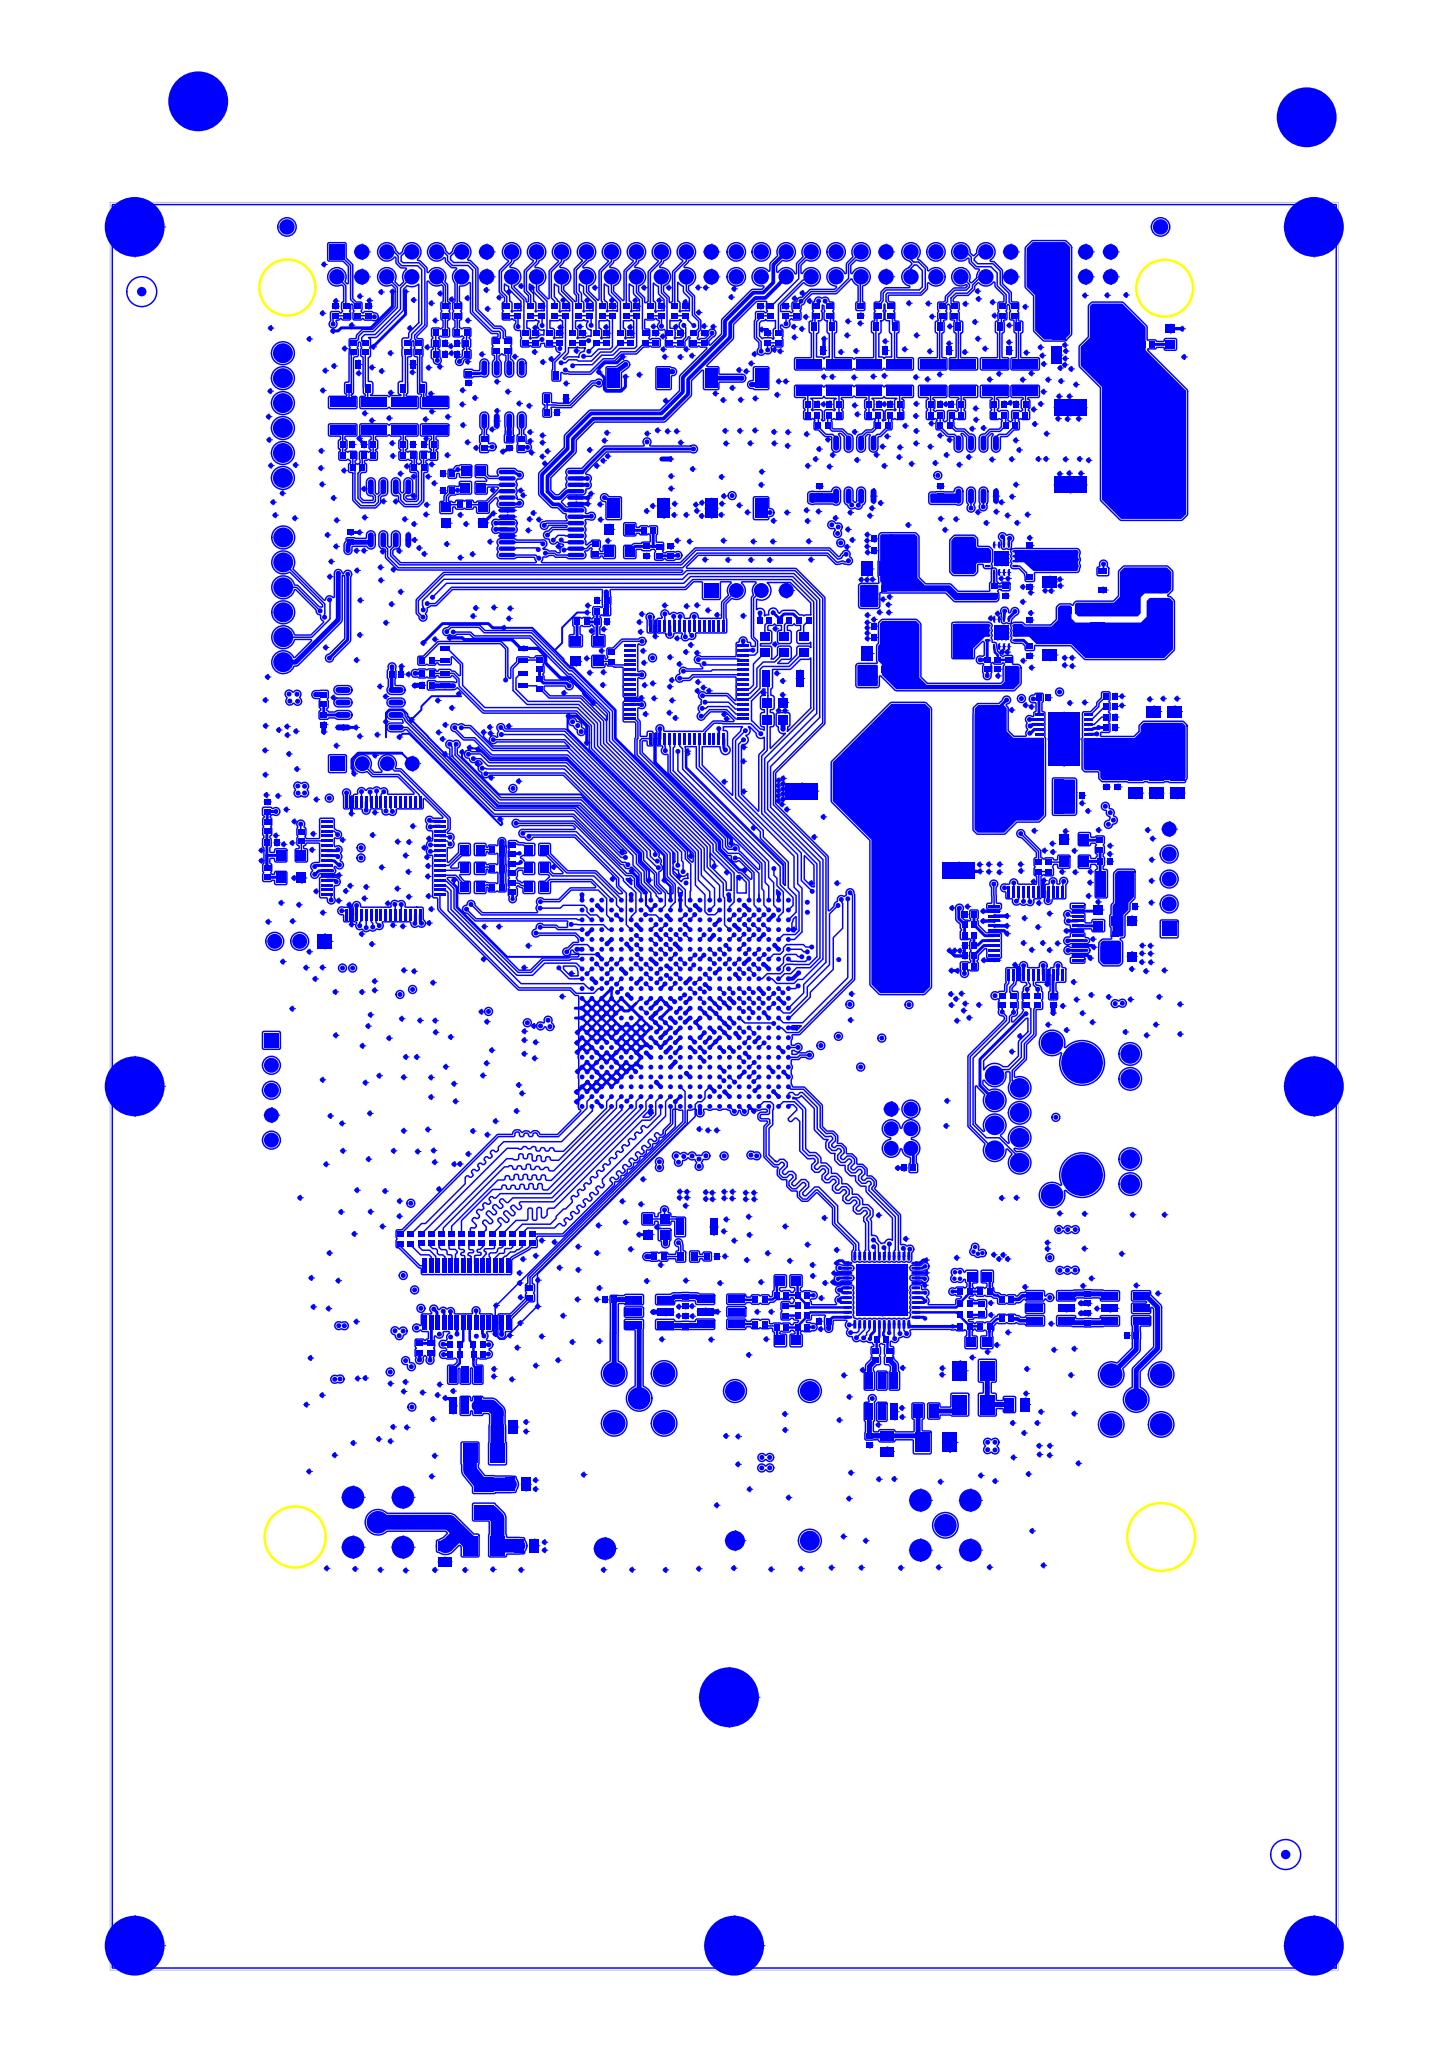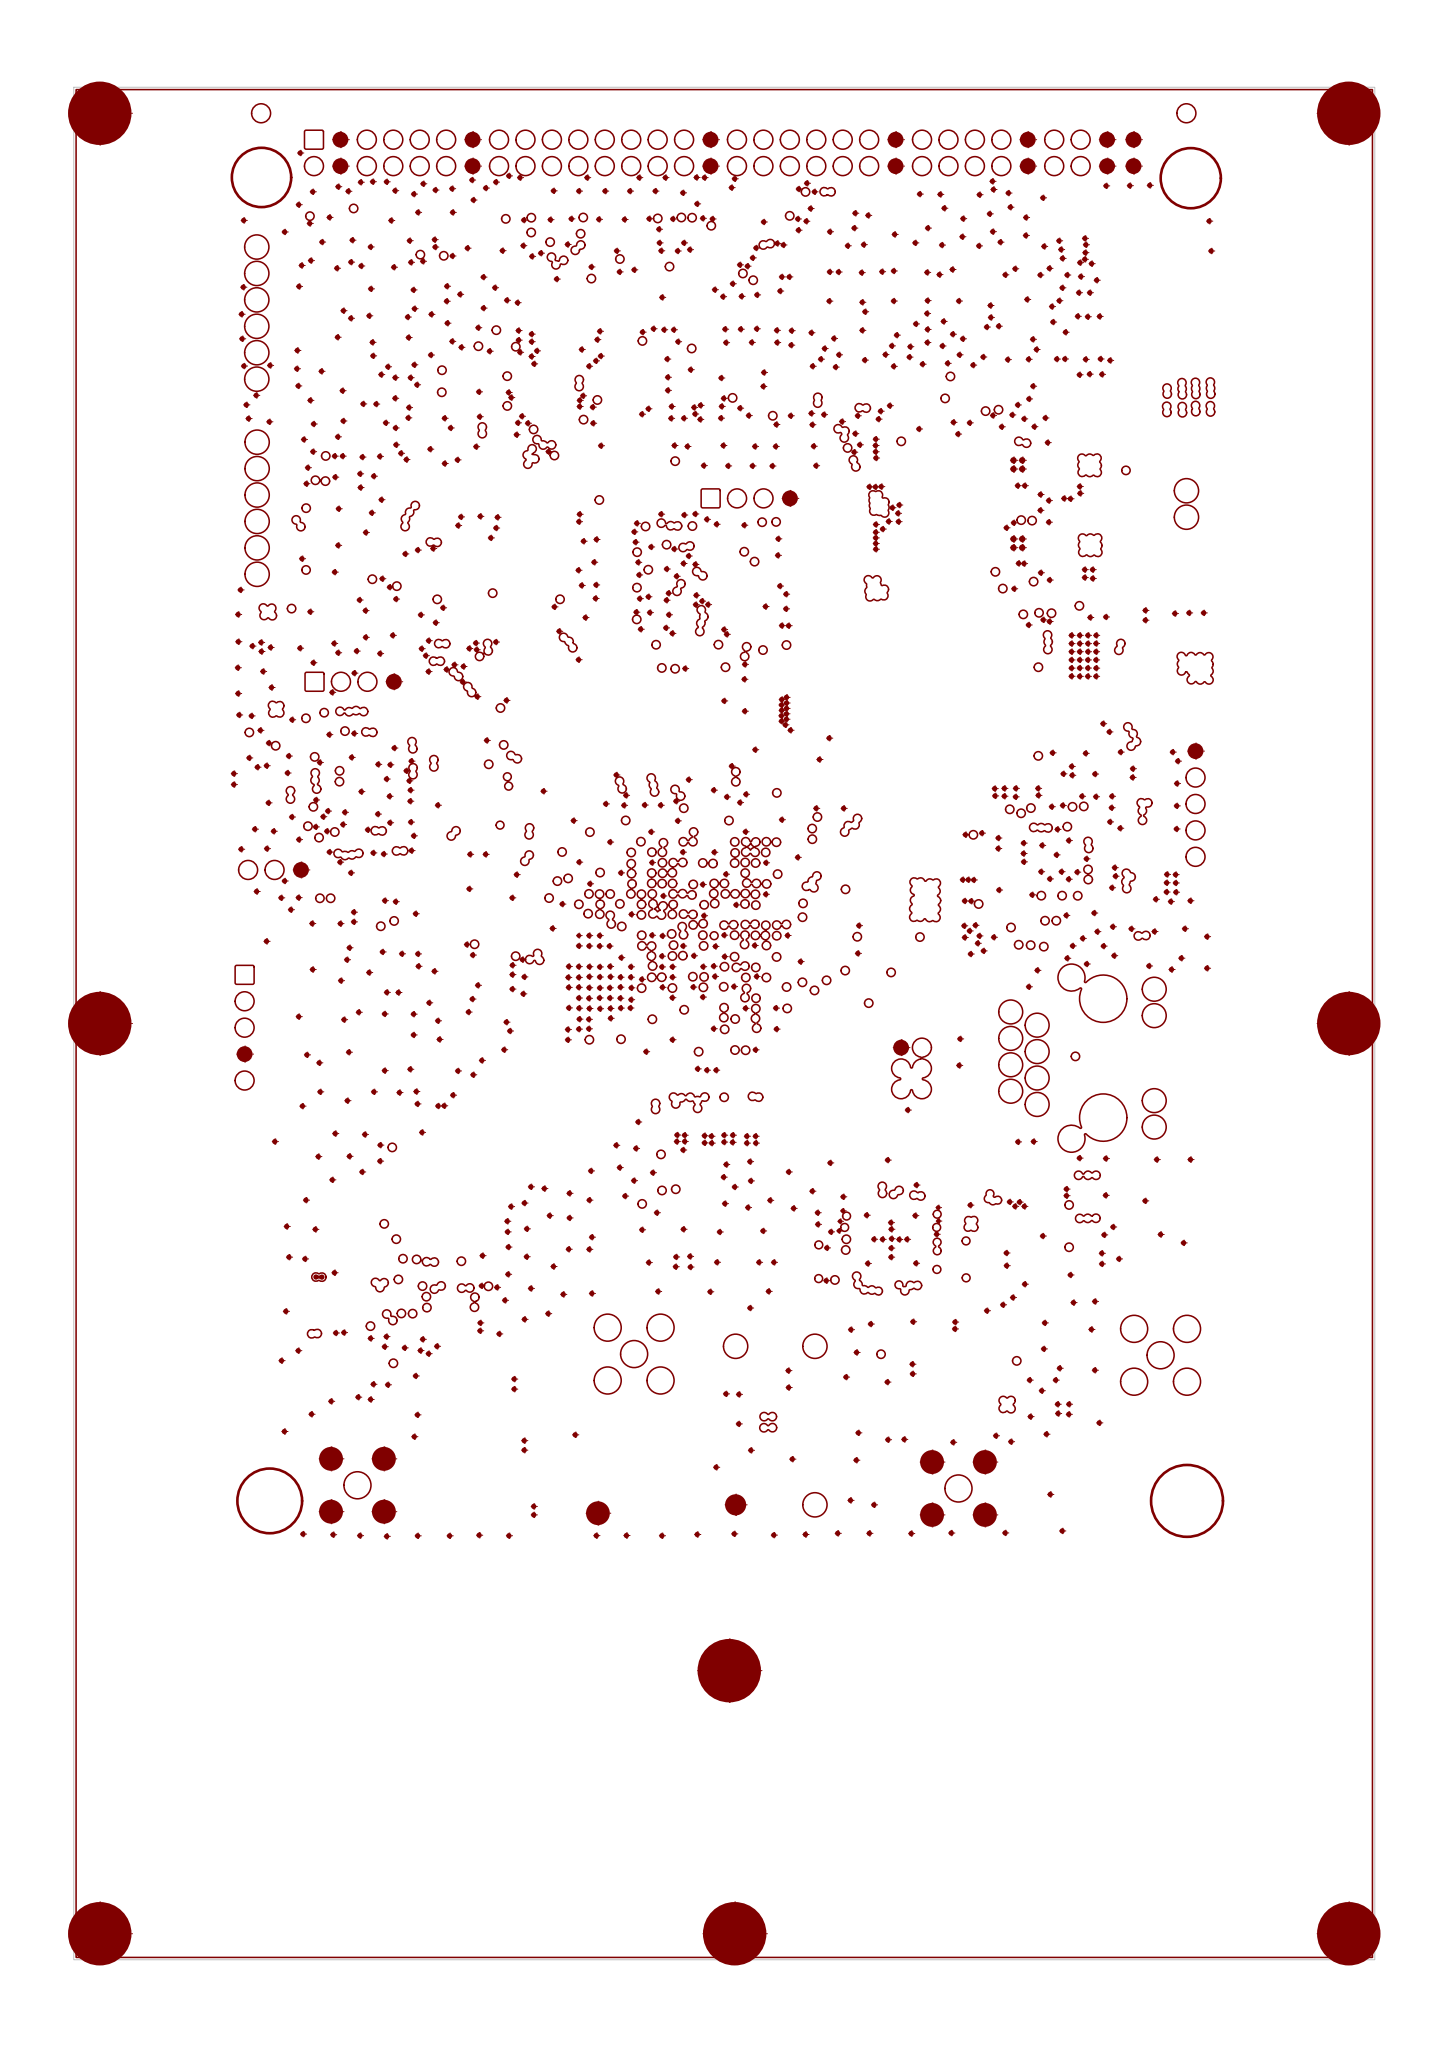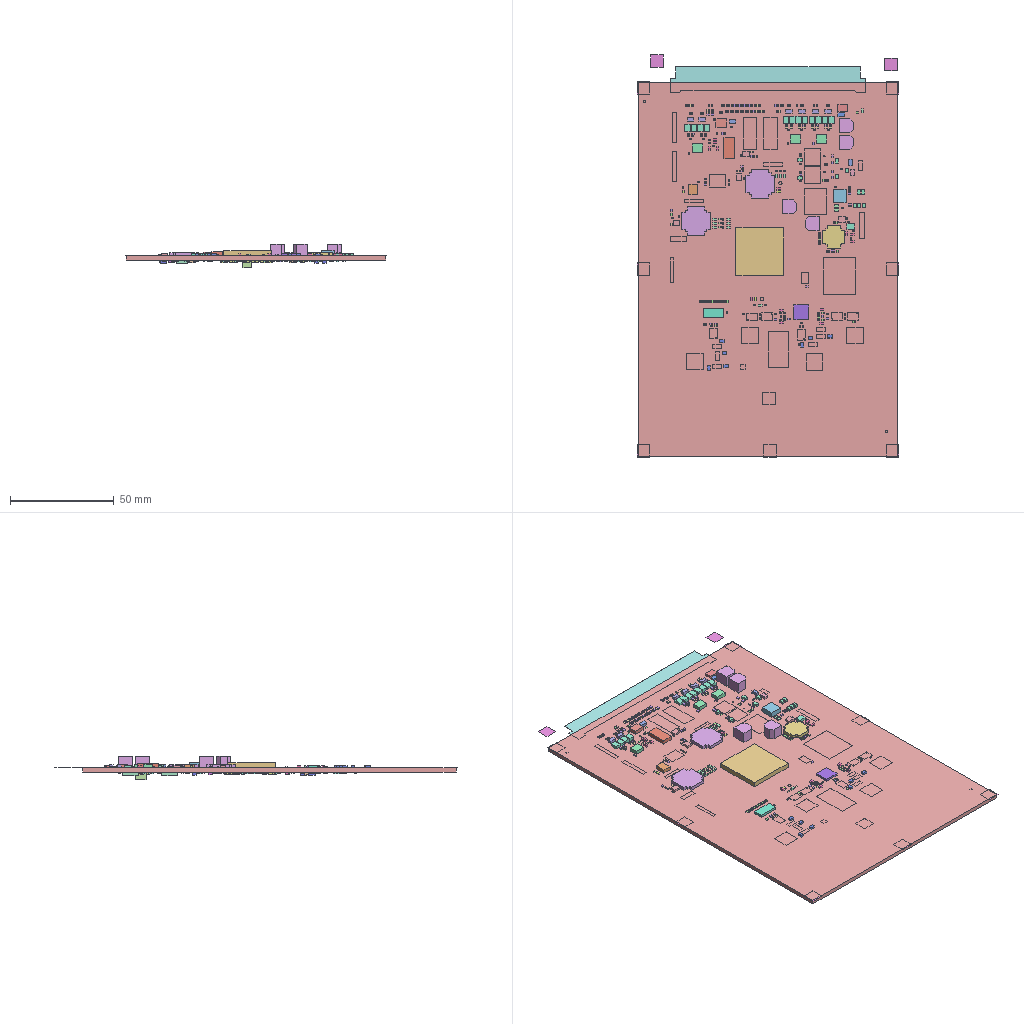Circuit board layout | Siemens PADS | box 126.1 x 193.9 x 11.1 mm
Layer stack:
layer,name,type,plane,layer_thickness_mm,copper_thickness_mm,dielectric_constant
0,,,,0,,3.3
1,Top,ROUTING,NONE,0.283,0.034,4.3
2,GND2,ROUTING,NONE,0.254,0.0351,4.3
3,SIG3,ROUTING,NONE,0.554,0.034,4.3
4,SIG4,ROUTING,NONE,0.2499,0.034,4.3
5,POWER5,ROUTING,NONE,0.4539,0.034,4.3
6,Bottom,ROUTING,NONE,0,0.034,3.3
Part placement, first 430 of 633 lines:
Ref,PartType,Decal,X_mm,Y_mm,Rotation,Layer,Placed,Installed
C1,CAP0805,CAPC1005X60N,30.658,-36.805,270,Bottom,True,True
C2,CAP0805,CAPC1005X60N,32.514,-101.452,270,Bottom,True,True
C3,CAP0805,CAPC2013X100L,40.208,-124.689,0,Top,True,True
C4,CAP0805,CAPC2013X100L,41.504,-130.531,0,Top,True,True
C5,CAP0805,CAPC2013X100L,42.367,-136.779,0,Top,True,True
C6,CAP0805,CAPC1608X90N,28.514,-117.318,90,Bottom,True,True
C7,CAP0805,CAPC1005X60N,70.622,-131.846,180,Bottom,True,True
C8,CAP0805,CAPC1005X60N,81.579,-126.895,270,Bottom,True,True
C9,CAP0805,CAPC1005X60N,77.069,-122.882,0,Bottom,True,True
C10,CAP0805,CAPC1005X60N,76.578,-131.624,270,Bottom,True,True
C11,CAP0805,CAPC2013X100L,92.32,-122.4,0,Top,True,True
C12,CAP0805,CAPC1608X90N,70.325,-123.37,180,Bottom,True,True
C13,CAP0805,CAPC1608X90N,70.336,-124.988,180,Bottom,True,True
C14,CAP0805,CAPC1608X90N,83.129,-126.57,270,Bottom,True,True
C15,CAP0805,CAPC1005X60N,88.724,-112.651,270,Top,True,True
C16,CAP0805,CAPC1005X60N,86.97,-114.46,0,Bottom,True,True
C17,CAP0805,CAPC1005X60N,91.239,-111.702,180,Top,True,True
C18,CAP0805,CAPC1608X90N,28.514,-121.876,270,Bottom,True,True
C19,CAP0805,CAPC1005X60N,30.067,-122.17,90,Bottom,True,True
C20,CAP0805,CAPC1005X60N,30.067,-116.806,270,Bottom,True,True
C21,CAP0805,CAPC1005X60N,32.527,-114.113,270,Bottom,True,True
C22,CAP0805,CAPC1005X60N,34.647,-114.113,270,Bottom,True,True
C23,CAP0805,CAPC1005X60N,37.277,-114.113,270,Bottom,True,True
C24,CAP0805,CAPC1005X60N,35.086,-116.297,180,Top,True,True
C25,CAP0805,CAPC1005X60N,37.466,-116.297,0,Top,True,True
C26,CAP0805,CAPC1608X90N,88.59,-27.07,270,Bottom,True,True
C27,CAP0805,CAPC1005X60N,87.157,-27.306,90,Bottom,True,True
C28,CAP0805,CAPC1005X60N,94.751,-27.414,90,Bottom,True,True
C29,CAP0805,CAPC2013X100L,34.036,-137.617,270,Top,True,True
C30,CAP0805,CAPC1005X60N,91.239,-113.684,180,Top,True,True
C31,CAP-AE4,CAPAE660X550N,100.29,-20.91,180,Top,True,True
C32,CAP0805,CAPC1005X60N,68.775,-11.06,270,Top,True,True
C33,CAP0805,CAPC1005X60N,54.57,-35.52,90,Top,True,True
C34,CAP0805,CAPC1005X60N,57.04,-35.52,270,Top,True,True
C35,CAP0805,CAPC1608X90N,54.76,-104.3,90,Top,True,True
C36,CAP0805,CAPC1005X60N,32.23,-49.174,180,Top,True,True
C37,CAP0805,CAPC1005X60N,98.675,-73.229,180,Bottom,True,True
C38,CAP0805,CAPC1005X60N,98.675,-75.007,180,Bottom,True,True
C39,CAP0805,CAPC1005X60N,55.43,-43.03,0,Bottom,True,True
C40,CAP0805,CAPC1005X60N,64.42,-43.38,270,Bottom,True,True
C41,CAP0805,CAPC1005X60N,52.783,-48.135,180,Bottom,True,True
C42,CAP0805,CAPC1005X60N,50.03,-42.72,180,Top,True,True
C43,CAP0805,CAPC1005X60N,50.03,-40.53,0,Top,True,True
C44,CAP0805,CAPC1005X60N,64.18,-45.59,180,Bottom,True,True
C45,CAP0805,CAPC1005X60N,61.21,-54.52,180,Bottom,True,True
C46,CAP0805,CAPC1005X60N,52.825,-51.147,180,Bottom,True,True
C47,CAP0805,CAPC1005X60N,63.18,-54.54,0,Bottom,True,True
C48,CAP0805,CAPC1608X90N,62.33,-43.84,180,Bottom,True,True
C49,CAP0805,CAPC1005X60N,84.462,-29.402,270,Top,True,True
C50,CAP0805,CAPC1005X60N,72.165,-29.402,270,Top,True,True
C51,CAP0805,CAPC1005X60N,73.681,-20.551,180,Top,True,True
C52,CAP0805,CAPC1005X60N,55.44,-54.57,180,Bottom,True,True
C53,CAP0805,CAPC1005X60N,71.491,-20.551,0,Top,True,True
C54,CAP0805,CAPC1005X60N,68.751,-112.863,270,Top,True,True
C55,CAP0805,CAPC1005X60N,77.917,-117.419,90,Top,True,True
C56,CAP0805,CAPC1005X60N,79.27,-117.419,90,Top,True,True
C57,CAP0805,CAPC1005X60N,79.854,-20.551,180,Top,True,True
C58,CAP0805,CAPC1005X60N,77.714,-20.551,0,Top,True,True
C59,CAP0805,CAPC1005X60N,24.497,-34.095,270,Top,True,True
C60,CAP0805,CAPC1005X60N,24.16,-24.657,0,Top,True,True
C61,CAP0805,CAPC1005X60N,26.3,-24.657,180,Top,True,True
C62,CAP0805,CAPC1005X60N,30.315,-24.657,0,Top,True,True
C63,CAP0805,CAPC1005X60N,32.445,-24.657,180,Top,True,True
C64,CAP0805,CAPC2013X100L,83.025,-123.064,0,Top,True,True
C65,CAP0805,CAPC2013X100L,79.046,-126.389,270,Top,True,True
C66,CAP0805,CAPC1005X60N,66.9,-13.81,270,Top,True,True
C67,CAP0805,CAPC1005X60N,56.087,-11.06,270,Top,True,True
C68,CAP0805,CAPC1005X60N,74.98,-110.03,270,Bottom,True,True
C69,CAP0805,CAPC1005X60N,74.98,-107.93,90,Bottom,True,True
C70,CAP0805,CAPC1005X60N,82,-107.96,90,Bottom,True,True
C71,CAP0805,CAPC1005X60N,82,-110.02,270,Bottom,True,True
C72,CAP0805,CAPC1005X60N,89.844,-110.018,270,Bottom,True,True
C73,CAP0805,CAPC1005X60N,98.233,-110.079,270,Bottom,True,True
C74,CAP0805,CAPC1608X90N,92.388,-110.297,90,Bottom,True,True
C75,CAP0805,CAPC1005X60N,90.96,-105.941,270,Bottom,True,True
C76,CAP0805,CAPC1005X60N,98.233,-106.056,270,Bottom,True,True
C77,CAP0805,CAPC1608X90N,92.388,-106.248,90,Bottom,True,True
C78,CAP0805,CAPC1005X60N,98.675,-76.082,180,Bottom,True,True
C79,CAP0805,CAPC1005X60N,96.391,-76.62,90,Bottom,True,True
C80,CAP0805,CAPC1005X60N,94.891,-76.62,90,Bottom,True,True
C81,CAP0805,CAPC1005X60N,92.933,-76.62,90,Bottom,True,True
C82,CAP0805,CAPC1608X90N,103.16,-73.154,180,Top,True,True
C83,CAP0805,CAPC1005X60N,98.675,-72.14,180,Bottom,True,True
C84,CAP0805,CAPC1608X90N,100.558,-72.842,270,Top,True,True
C85,CAP0805,CAPC1005X60N,101.239,-67.1,180,Top,True,True
C86,CAP0805,CAPC1005X60N,103.808,-71.702,180,Top,True,True
C87,CAP0805,CAPC1005X60N,95,-70.37,0,Bottom,True,True
C88,CAP0805,CAPC1005X60N,95.77,-95.24,0,Bottom,True,True
C89,CAP0805,CAPC1005X60N,93.296,-81.246,270,Top,True,True
C90,CAP0805,CAPC1005X60N,94.424,-81.246,270,Top,True,True
C91,CAP0805,CAPC1005X60N,86.382,-91.479,0,Bottom,True,True
C92,CAP0805,CAPC1608X90N,103.16,-76.79,180,Top,True,True
C93,CAP0805,CAPC1005X60N,58.543,-11.06,270,Top,True,True
C94,CAP0805,CAPC1005X60N,58.024,-13.81,270,Top,True,True
C95,CAP0805,CAPC1005X60N,86.112,-20.551,180,Top,True,True
C96,CAP0805,CAPC1005X60N,60.454,-13.81,270,Top,True,True
C97,CAP0805,CAPC1005X60N,55.51,-13.81,270,Top,True,True
C98,CAP0805,CAPC1005X60N,53.582,-11.06,270,Top,True,True
C99,CAP0805,CAPC1005X60N,83.982,-20.551,0,Top,True,True
C100,CAP0805,CAPC1005X60N,52.989,-13.81,270,Top,True,True
C101,CAP0805,CAPC1005X60N,92.668,-20.551,180,Top,True,True
C102,CAP0805,CAPC1005X60N,90.487,-20.551,0,Top,True,True
C103,CAP0805,CAPC1005X60N,51.119,-11.06,270,Top,True,True
C104,CAP0805,CAPC1608X90N,99.43,-54.92,90,Bottom,True,True
C105,CAP0805,CAPC1608X90N,101.73,-54.26,90,Bottom,True,True
C106,CAP0805,CAPC1005X60N,101.803,-53.491,0,Top,True,True
C107,CAP0805,CAPC1005X60N,50.543,-13.81,270,Top,True,True
C108,CAP0805,CAPC1005X60N,48.752,-11.06,270,Top,True,True
C109,CAP0805,CAPC1005X60N,48.09,-13.81,270,Top,True,True
C110,CAP0805,CAPC1005X60N,46.341,-11.06,270,Top,True,True
C111,CAP0805,CAPC1005X60N,45.72,-13.81,270,Top,True,True
C112,CAP0805,CAPC1005X60N,23.719,-37.168,180,Bottom,True,True
C113,CAP0805,CAPC1005X60N,63.897,-124.312,270,Bottom,True,True
C114,CAP0805,CAPC1005X60N,43.872,-11.06,270,Top,True,True
C115,CAP0805,CAPC1005X60N,43.328,-13.81,270,Top,True,True
C116,CAP0805,CAPC1005X60N,22.904,-11.06,270,Top,True,True
C117,CAP0805,CAPC1005X60N,41.45,-11.06,270,Top,True,True
C118,CAP0805,CAPC1005X60N,26.278,-11.06,270,Top,True,True
C119,CAP0805,CAPC1005X60N,66.16,-11.06,270,Top,True,True
C120,CAP0805,CAPC1005X60N,104.883,-71.281,0,Bottom,True,True
C121,CAP0805,CAPC1005X60N,104.883,-69.086,0,Bottom,True,True
C122,CAP0805,CAPC1005X60N,104.883,-66.89,0,Bottom,True,True
C123,CAP0805,CAPC2013X120N,106.21,-52.745,90,Top,True,True
C124,CAP0805,CAPC2013X120N,108.577,-59.248,270,Top,True,True
C125,CAP0805,CAPC2013X120N,106.44,-59.248,270,Top,True,True
C126,CAP0805,CAPC2013X120N,104.37,-59.248,270,Top,True,True
C127,CAP0805,CAPC2013X120N,108.311,-52.745,90,Top,True,True
C128,CAP0805,CAPC1005X60N,101.36,-59.03,270,Top,True,True
C129,CAP0805,CAPC1005X60N,102.56,-59.03,270,Top,True,True
C130,CAP0805,CAPC1005X60N,23.826,-28.468,270,Bottom,True,True
C131,CAP0805,CAPC1005X60N,104.883,-64.771,0,Bottom,True,True
C132,CAP-AE4,CAPAE660X550N,100.29,-28.77,180,Top,True,True
C133,CAP0805,CAPC1608X90N,67.68,-50.93,180,Top,True,True
C134,CAP0805,CAPC2013X120N,51.219,-70.341,0,Bottom,True,True
C135,CAP0805,CAPC1608X90N,47.44,-77.25,180,Bottom,True,True
C136,CAP0805,CAPC1005X60N,52.46,-77.18,90,Bottom,True,True
C137,CAP0805,CAPC1005X60N,49.467,-80.469,270,Bottom,True,True
C138,CAP0805,CAPC1005X60N,49.575,-74.904,0,Bottom,True,True
C139,CAP0805,CAPC2013X120N,47.78,-71.72,0,Bottom,True,True
C140,CAP0805,CAPC1608X90N,67.29,-79.37,0,Bottom,True,True
C141,CAP0805,CAPC1005X60N,68.1,-74.83,180,Bottom,True,True
C142,CAP0805,CAPC1005X60N,63.754,-76.352,90,Bottom,True,True
C143,CAP0805,CAPC1005X60N,67.7,-82.3,180,Bottom,True,True
C144,CAP0805,CAPC2013X120N,62.125,-69.359,0,Bottom,True,True
C145,CAP0805,CAPC1608X90N,68.39,-77.57,180,Bottom,True,True
C146,CAP0805,CAPC1005X60N,59.21,-78.67,180,Bottom,True,True
C147,CAP0805,CAPC1005X60N,60.76,-77.39,90,Bottom,True,True
C148,CAP0805,CAPC1005X60N,63.07,-82.31,0,Bottom,True,True
C149,CAP0805,CAPC2013X120N,56.63,-70.85,90,Bottom,True,True
C150,CAP0805,CAPC1608X90N,59.11,-75.48,0,Bottom,True,True
C151,CAP0805,CAPC1005X60N,55.79,-80.65,270,Bottom,True,True
C152,CAP0805,CAPC1005X60N,54.67,-76.29,90,Bottom,True,True
C153,CAP0805,CAPC1005X60N,52.966,-72.902,0,Bottom,True,True
C154,CAP0805,CAPC2013X120N,61.25,-92.46,270,Bottom,True,True
C155,CAP0805,CAPC1608X90N,66.6,-91.48,0,Bottom,True,True
C156,CAP0805,CAPC1005X60N,61.56,-80.38,90,Bottom,True,True
C157,CAP0805,CAPC1005X60N,68.05,-89.33,0,Bottom,True,True
C158,CAP0805,CAPC1005X60N,65.95,-86.82,180,Bottom,True,True
C159,CAP0805,CAPC2013X120N,69.24,-87.52,180,Bottom,True,True
C160,CAP0805,CAPC1608X90N,53.08,-82.38,145,Bottom,True,True
C161,CAP0805,CAPC1005X60N,61.53,-89.35,270,Bottom,True,True
C162,CAP0805,CAPC1005X60N,59.58,-82.05,270,Bottom,True,True
C163,CAP0805,CAPC1005X60N,57.27,-80.46,0,Bottom,True,True
C164,CAP0805,CAPC1005X60N,53.772,-80.34,180,Bottom,True,True
C165,CAP0805,CAPC1005X60N,56.29,-87.32,0,Bottom,True,True
C166,CAP0805,CAPC1608X90N,65.19,-83.4,0,Bottom,True,True
C167,CAP0805,CAPC1005X60N,58.76,-85.86,270,Bottom,True,True
C168,CAP0805,CAPC1005X60N,61.22,-83.42,180,Bottom,True,True
C169,CAP0805,CAPC1005X60N,54.534,-83.769,0,Bottom,True,True
C170,CAP0805,CAPC1005X60N,54.55,-85.02,0,Bottom,True,True
C171,CAP0805,CAPC1005X60N,63.001,-85.345,180,Bottom,True,True
C172,CAP0805,CAPC1005X60N,56.67,-82.63,45,Bottom,True,True
C173,CAP0805,CAPC1005X60N,59.22,-84.3,0,Bottom,True,True
C174,CAP0805,CAPC1005X60N,81.25,-98.31,180,Top,True,True
C175,CAP0805,CAPC1005X60N,79.93,-83.99,0,Bottom,True,True
C176,CAP0805,CAPC1005X60N,79.93,-81.69,180,Bottom,True,True
C177,CAP0805,CAPC1005X60N,56.67,-88.4,180,Bottom,True,True
C178,CAP0805,CAPC1005X60N,58.64,-90.89,90,Bottom,True,True
C179,CAP0805,CAPC1005X60N,33.611,-15.455,180,Top,True,True
C180,CAP0805,CAPC1005X60N,35.801,-15.459,0,Top,True,True
C203,CAP0805,CAPC1005X60N,92.738,-49.408,270,Bottom,True,True
C204,CAP0805,CAPC1005X60N,93.838,-49.408,90,Bottom,True,True
C207,CAP0805,CAPC2013X120N,62.47,-87.46,180,Bottom,True,True
C208,CAP0805,CAPC1005X60N,24.128,-17.841,270,Bottom,True,True
C209,CAP0805,CAPC2013X120N,58.85,-98.85,270,Bottom,True,True
C210,CAP0805,CAPC2013X120N,84.97,-77.2,180,Bottom,True,True
C211,CAP0805,CAPC1005X60N,89.844,-105.941,270,Bottom,True,True
C212,CAP0805,CAPC1005X60N,90.96,-110.018,270,Bottom,True,True
C213,CAP0805,CAPC1005X60N,16.98,-50.77,0,Bottom,True,True
C214,CAP0805,CAPC1005X60N,17.809,-58.361,180,Bottom,True,True
C215,CAP0805,CAPC1608X90N,18.11,-56.9,0,Bottom,True,True
C219,CAP0805,CAPC2013X120N,84.97,-73.04,180,Bottom,True,True
C220,CAP0805,CAPC2013X120N,84.95,-75.13,180,Bottom,True,True
C221,CAP0805,CAPC2013X120N,63.095,-98.82,270,Bottom,True,True
C254,CAP0805,CAPC1005X60N,78.247,-43.156,180,Top,True,True
C255,CAP0805,CAPC1005X60N,93.594,-43.022,90,Top,True,True
C256,CAP0805,CAPC1005X60N,93.594,-45.68,90,Top,True,True
C257,CAP0805,CAPC1005X60N,78.247,-44.311,180,Top,True,True
C266,CAP0805,CAPC2013X120N,65.22,-98.84,270,Bottom,True,True
C271,CAP0805,CAPC2013X120N,61,-98.827,270,Bottom,True,True
C272,CAP0805,CAPC2013X120N,95.631,-45.191,270,Top,True,True
C273,CAP0805,CAPC2013X120N,77.974,-45.937,180,Top,True,True
C280,CAP-AE4,CAPAE660X550N,83.759,-67.999,0,Top,True,True
C281,CAP0805,CAPC1005X60N,21.742,-52.68,270,Top,True,True
C282,CAP0805,CAPC1005X60N,29.14,-48.04,0,Top,True,True
C283,CAP0805,CAPC1005X60N,16.408,-98.527,90,Bottom,True,True
C284,CAP0805,CAPC1608X90N,66.17,-28.11,180,Bottom,True,True
C285,CAP0805,CAPC1005X60N,24.53,-61.11,0,Bottom,True,True
C286,CAP0805,CAPC1005X60N,22.05,-68.68,270,Bottom,True,True
C287,CAP0805,CAPC1005X60N,22.093,-65.676,180,Bottom,True,True
C288,CAP0805,CAPC1005X60N,16.443,-65.195,180,Top,True,True
C289,CAP0805,CAPC1005X60N,15.988,-61.531,270,Top,True,True
C290,CAP0805,CAPC1005X60N,33.3,-64.2,90,Bottom,True,True
C291,CAP0805,CAPC1005X60N,30.29,-72.56,180,Bottom,True,True
C292,CAP0805,CAPC1005X60N,24.49,-70.83,180,Bottom,True,True
C293,CAP0805,CAPC1005X60N,32.32,-72.56,0,Bottom,True,True
C294,CAP0805,CAPC1608X90N,31,-61.448,180,Bottom,True,True
C295,CAP0805,CAPC1005X60N,40.602,-24.538,270,Top,True,True
C316,CAP0805,CAPC2013X120N,50.591,-90.505,90,Bottom,True,True
C317,CAP0805,CAPC1608X90N,52.605,-89.948,270,Bottom,True,True
C318,CAP0805,CAPC1005X60N,59.59,-88.19,90,Bottom,True,True
C319,CAP0805,CAPC1005X60N,54.51,-89.21,0,Bottom,True,True
C320,CAP0805,CAPC1005X60N,54.312,-87.077,0,Bottom,True,True
C348,CAP0805,CAPC1005X60N,78.247,-34.27,180,Top,True,True
C349,CAP0805,CAPC1005X60N,93.594,-35.418,90,Top,True,True
C350,CAP0805,CAPC1005X60N,93.594,-38.654,90,Top,True,True
C351,CAP0805,CAPC1005X60N,31.298,-62.754,180,Bottom,True,True
C352,CAP0805,CAPC1005X60N,78.247,-35.468,180,Top,True,True
C353,CAP0805,CAPC2013X120N,95.631,-37.735,270,Top,True,True
C354,CAP0805,CAPC2013X120N,77.974,-37.324,180,Top,True,True
C355,CAP-AE4,CAPAE660X550N,72.978,-59.946,180,Top,True,True
C356,CAP0805,CAPC1005X60N,92.681,-56.906,90,Bottom,True,True
C357,CAP0805,CAPC1005X60N,98.417,-60.405,180,Top,True,True
C359,CAP0805,CAPC1005X60N,98.02,-41.52,0,Top,True,True
C360,CAP0805,CAPC2013X120N,100.47,-42.42,90,Top,True,True
C362,CAP0805,CAPC1005X60N,70.47,-114.54,180,Bottom,True,True
C364,CAP0805,CAPC1005X60N,66.165,-111.71,0,Top,True,True
C365,CAP0805,CAPC1005X60N,66.165,-114.207,0,Top,True,True
C366,CAP0805,CAPC1005X60N,84.2,-110.89,180,Bottom,True,True
C367,CAP0805,CAPC1005X60N,84.2,-111.99,180,Bottom,True,True
C368,CAP0805,CAPC1005X60N,82,-113.02,90,Bottom,True,True
C369,CAP0805,CAPC1005X60N,73.28,-112.26,270,Bottom,True,True
C370,CAP0805,CAPC1005X60N,76.98,-114.38,0,Bottom,True,True
C371,CAP0805,CAPC1005X60N,72.644,-113.917,180,Top,True,True
C372,CAP0805,CAPC1005X60N,74.98,-112.3,270,Bottom,True,True
C373,CAP0805,CAPC1005X60N,72.97,-110.74,0,Bottom,True,True
C374,CAP0805,CAPC1005X60N,79.79,-114.38,180,Bottom,True,True
C466,CAP0805,CAPC2013X120N,46.64,-23.87,0,Bottom,True,True
C467,CAP0805,CAPC1608X90N,46.64,-27.66,180,Bottom,True,True
C468,CAP0805,CAPC1608X90N,46.64,-25.81,0,Bottom,True,True
C469,CAP0805,CAPC1608X90N,40.862,-32.35,180,Bottom,True,True
C470,CAP0805,CAPC1608X90N,40.081,-30.582,180,Bottom,True,True
C471,CAP0805,CAPC1608X90N,40.862,-33.949,180,Bottom,True,True
C472,CAP0805,CAPC1608X90N,59.03,-93.53,270,Bottom,True,True
C473,CAP0805,CAPC1608X90N,46.64,-29.46,180,Bottom,True,True
C474,CAP0805,CAPC1608X90N,40.081,-27.842,0,Bottom,True,True
C475,CAP0805,CAPC1608X90N,34.209,-31.865,90,Top,True,True
C476,CAP0805,CAPC1608X90N,37.938,-31.832,270,Top,True,True
C477,CAP0805,CAPC1608X90N,36.962,-29.054,180,Top,True,True
C478,CAP0805,CAPC1608X90N,36.976,-27.37,180,Top,True,True
C479,CAP0805,CAPC2013X120N,67.43,-30.01,0,Bottom,True,True
C480,CAP0805,CAPC2013X120N,51.023,-28.302,270,Bottom,True,True
C481,CAP0805,CAPC1005X60N,68.787,-25.479,180,Bottom,True,True
C482,CAP0805,CAPC1005X60N,62.746,-26.148,270,Bottom,True,True
C483,CAP0805,CAPC1005X60N,62.746,-28.25,270,Bottom,True,True
C484,CAP0805,CAPC1005X60N,55.905,-24.587,0,Bottom,True,True
C485,CAP0805,CAPC1005X60N,52.701,-27.51,270,Bottom,True,True
C486,CAP0805,CAPC2013X120N,52.59,-31.53,0,Bottom,True,True
C487,CAP0805,CAPC2013X120N,60.24,-24.1,0,Bottom,True,True
D1,XC7A75,BGA484C100P22X22_2300X2300X244,58.528,-81.549,90,Top,True,True
D2,ADC3244,QFN50P700X700X100-49AN,78.534,-110.766,0,Top,True,True
D3,W25Q256FVE,WSON8,38.048,-47.318,180,Top,True,True
D4,W5500,LQFP48-7X7MM,94.206,-74.416,90,Top,True,True
D5,STM32F4X5RG,LQFP64-10X10MM,58.702,-48.846,0,Top,True,True
D6,SP3490EN,SOIC127P600X180-8N,88.244,-27.209,90,Top,True,True
D7,RJGT102,SOIC127P600X180-8N,26.398,-51.554,0,Top,True,True
D8,SM712,SOT95P285X140-3L,85.37,-13.888,270,Top,True,True
D9,SM712,SOT95P285X140-3L,91.485,-13.888,270,Top,True,True
D10,STM32F4X5RG,LQFP64-10X10MM,27.814,-66.759,0,Top,True,True
D11,SP3490EN,SOIC127P600X180-8N,75.786,-27.209,90,Top,True,True
D12,SM712,SOT95P285X140-3L,72.537,-13.888,270,Top,True,True
D13,SM712,SOT95P285X140-3L,78.879,-13.888,270,Top,True,True
D14,SP3490EN,SOIC127P600X180-8N,28.439,-31.667,90,Top,True,True
D15,SM712,SOT95P285X140-3L,25.266,-17.711,90,Top,True,True
D16,SM712,SOT95P285X140-3L,30.791,-17.711,90,Top,True,True
D24,ADUM3151,SOP65P790X185-20N,27.012,-41.947,0,Bottom,True,True
D25,PCA82C250,SOIC127P600X180-8N,39.984,-19.567,90,Top,True,True
D28,ADUM3151,SOP65P790X185-20N,26.652,-23.083,180,Bottom,True,True
E1,ESP_WROOM_02,ESP_WROOM_02U,33.967,-99.195,90,Bottom,True,True
E2,ATK1218,ATK1218,16.416,-90.401,270,Top,True,True
FB1,RES0805,RESC1005X40N,55.869,-35.52,90,Top,True,True
FB2,RES0805,RESC1005X40N,88.756,-110.018,90,Bottom,True,True
FB3,RES0805,RESC1005X40N,102.356,-74.985,90,Top,True,True
FB4,RES0805,RESC1005X40N,88.756,-105.941,90,Bottom,True,True
FB5,RES0805,RESC1005X40N,50.03,-41.63,180,Top,True,True
FB53,RES0805,RESC1005X40N,15.988,-63.569,270,Top,True,True
FB54,RES0805,RESC1005X40N,57.17,-89.94,90,Bottom,True,True
J1,CON-SIP-5P,SIP-5P,107.777,-73.976,90,Top,True,True
J2,CON-SIP-3P,SIP-3P,21.832,-75.239,180,Top,True,True
J3,SMA,SMA_KE_A,27.258,-134.388,0,Top,True,True
J4,SMA,SMA_KE_A,85.002,-134.697,90,Top,True,True
J5,CON-SIP-6P,MOLEX_5267_6P,17.618,-46.818,90,Top,True,True
J6,CON-SIP-6P,MOLEX_5267_6P,17.585,-28.058,90,Top,True,True
J7,SMA,SMA_KE_A,104.419,-121.891,0,Top,True,True
J10,CON-SIP-6P,FPGA_JTAG,81.49,-96.32,90,Top,True,True
J11,CON-SIP-2P,MOLEX_5267_2P,106.906,-41.327,90,Top,True,True
J17,CON-41612-64B,DIN41612-64B,18,-2.5,0,Top,False,True
J20,SMA,SMA_KE_A,53.839,-121.776,0,Top,True,True
L1,IND-UPRIGHT,INDUCT_HC0630,83.907,-44.614,180,Top,True,True
L2,IND-UPRIGHT,CDRH3D16,26.108,-122.692,90,Bottom,True,True
L3,IND-UPRIGHT,CDRH3D16,26.108,-116.906,90,Bottom,True,True
L4,IND-UPRIGHT,CDRH3D16,71.098,-128.458,90,Bottom,True,True
L5,IND-MOLDED,IND-1008,38.024,-127.381,180,Top,True,True
L6,IND-MOLDED,IND-1008,38.049,-131.953,270,Top,True,True
L7,IND-MOLDED,IND-1008,38.034,-136.755,180,Top,True,True
L8,IND-MOLDED,INDC3225X135L,102.271,-69.371,0,Top,True,True
L9,IND-UPRIGHT,INDUCT_HC0630,83.907,-35.95,180,Top,True,True
L10,IND-MOLDED,INDC3225X135L,83.709,-17.841,90,Top,True,True
L11,IND-UPRIGHT,IN07175,85.523,-57.432,180,Top,True,True
L12,IND-UPRIGHT,CDRH3D16,88.121,-125.516,90,Bottom,True,True
L13,IND-MOLDED,INDC3225X135L,86.843,-17.841,90,Top,True,True
L14,IND-MOLDED,IND-1008,87.87,-122.411,180,Top,True,True
L15,IND-MOLDED,IND-1008,87.87,-118.96,0,Top,True,True
L16,IND-MOLDED,IND-1008,84.043,-126.263,180,Top,True,True
L17,IND-MOLDED,INDC3225X135L,71.1,-17.841,90,Top,True,True
L18,IND-MOLDED,INDC3225X135L,74.181,-17.841,90,Top,True,True
L19,INDUCT_1,INDC1608X95N,88.465,-109.374,180,Top,True,True
L20,INDUCT_1,INDC1608X95N,88.416,-116.069,180,Top,True,True
L21,INDUCT_1,INDC1608X95N,69,-109.84,0,Top,True,True
L22,INDUCT_1,INDC1608X95N,69.01,-115.88,0,Top,True,True
L23,IND-MOLDED,INDC3225X135L,77.232,-17.841,90,Top,True,True
L24,IND-MOLDED,INDC3225X135L,90.008,-17.841,90,Top,True,True
L25,IND-MOLDED,INDC3225X135L,80.302,-17.841,90,Top,True,True
L26,IND-MOLDED,INDC3225X135L,26.862,-21.773,90,Top,True,True
L27,IND-MOLDED,INDC3225X135L,23.672,-21.773,90,Top,True,True
L28,IND-MOLDED,INDC3225X135L,93.118,-17.841,90,Top,True,True
L29,IND-MOLDED,INDC3225X135L,33.022,-21.773,90,Top,True,True
L30,IND-MOLDED,INDC3225X135L,29.902,-21.773,90,Top,True,True
LED1,LED,LEDC1608X80N,36.858,-65.89,180,Top,True,True
LED2,LED,LEDC1608X80N,36.858,-67.81,180,Top,True,True
LED3,LED,LEDC1608X80N,36.858,-69.748,180,Top,True,True
LED4,LED,LEDC1608X80L,74.16,-86.54,90,Bottom,True,True
LED5,LED,LEDC1608X80N,43.417,-65.89,0,Top,True,True
LED6,LED,LEDC1608X80N,43.417,-69.748,0,Top,True,True
LED7,LED,LEDC1608X80N,43.417,-67.81,0,Top,True,True
LED8,LED,LEDC1608X80L,58.776,-107.333,0,Top,True,True
LED9,LED,LEDC1608X80N,66.635,-45.051,270,Top,True,True
LED10,LED,LEDC1608X80N,107.9,-13.66,90,Top,True,True
LED11,LED,LEDC1608X80N,68.621,-45.051,270,Top,True,True
LED12,LED,LEDC1608X80N,70.581,-45.051,270,Top,True,True
M1,SCREWHOLE_M3,SCREWHOLE_M3,122.5,-90,0,Top,False,True
M2,SCREWHOLE_M3,SCREWHOLE_M3,63.5,-177.5,0,Top,False,True
M3,SCREWHOLE_M3,SCREWHOLE_M3,2.5,-177.5,0,Top,False,True
M4,SCREWHOLE_M3,SCREWHOLE_M3,122.5,-177.5,0,Top,False,True
M5,SCREWHOLE_M3,SCREWHOLE_M3,2.5,-90,0,Top,False,True
M6,SCREWHOLE_M3,SCREWHOLE_M3,62.98,-152.21,0,Top,True,True
M7,MARK,MARK,7.03,-167.8,0,Bottom,True,True
M8,MARK,MARK,3.22,-9.09,0,Top,True,True
M9,MARK,MARK,119.63,-168.22,0,Top,True,True
M10,MARK,MARK,121.63,-9.22,0,Bottom,True,True
M11,GNDPOINT,GND_POINT,50.362,-137.074,0,Top,True,True
M12,SCREWHOLE_M3,SCREWHOLE_M3,2.5,-2.5,0,Top,False,True
M13,SCREWHOLE_M3,SCREWHOLE_M3,8.966,10.287,0,Top,False,True
M14,SCREWHOLE_M3,SCREWHOLE_M3,121.768,8.661,0,Top,False,True
M15,SCREWHOLE_M3,SCREWHOLE_M3,122.5,-2.5,0,Top,False,True
N1,SPX3819M5,SOT95P280X145-5N,95.379,-110.551,0,Bottom,True,True
N2,DAC904E,SOP65P640X120-28N,36.267,-111.173,270,Top,True,True
N3,SPX3819M5,SOT95P280X145-5N,95.379,-106.501,0,Bottom,True,True
N4,NMOS,SOT95P285X140-3L,45.415,-18.796,90,Top,True,True
N5,TPS53355,DQP22_5P479X3P24,97.04,-54.655,0,Top,True,True
N6,SPX3819M5,SOT95P280X145-5N,91.732,-28.831,0,Bottom,True,True
N8,TLV62130RGT,RGT0016A,90.709,-43.841,0,Top,True,True
N10,NMOS,SOT95P285X140-3L,21.687,-61.786,90,Bottom,True,True
N12,NMOS,SOT95P285X140-3L,102.228,-38.519,0,Top,True,True
N20,TLV62130RGT,RGT0016A,90.708,-36.278,0,Top,True,True
N22,SPX3819M5,SOT95P280X145-5N,17.99,-53.84,270,Bottom,True,True
N35,WM8510,SOP65P780X200-28AN,43.901,-31.683,0,Top,True,True
N37,OPA1612,SOIC127P594X363-8N,58.31,-28.04,0,Bottom,True,True
OSC1,JZ,OSCSC210P250X320X110-4L,51.84,-34.44,270,Top,True,True
OSC2,JZ,TCXO_DIP14,63.59,-121.028,0,Top,True,True
OSC3,JZ,OSCSC210P250X320X110-4L,98.102,-65.983,270,Top,True,True
OSC4,JZ,OSCSC210P250X320X110-4L,18.414,-67.639,90,Top,True,True
OSC5,JZ,OSCSC210P250X320X110-4L,48.54,-45.69,0,Top,True,True
Q1,MMBT3904LT1,SOT23,77.574,-126.558,90,Bottom,True,True
R1,RES0805,RESC1005X40N,39.334,-14.644,90,Top,True,True
R2,RES0805,RESC1005X40N,40.394,-14.634,90,Top,True,True
R3,RES0805,RESC1005X40N,54.79,-33.39,0,Top,True,True
R4,RES0805,RESC1005X40N,49.42,-35.3,270,Top,True,True
R5,RES0805,RESC1005X40N,31.195,-101.452,270,Bottom,True,True
R6,RES0805,RESC1005X40N,26.508,-101.452,90,Bottom,True,True
R7,RES0805,RESC1005X40N,23.506,-101.452,90,Bottom,True,True
R8,RES0805,RESC1005X40N,25.881,-79.004,270,Bottom,True,True
R9,RES0805,RESC1005X40N,22.439,-79.004,270,Bottom,True,True
R10,RES0805,RESC1005X40N,24.771,-79.004,270,Bottom,True,True
R11,RES0805,RESC1005X40N,23.552,-79.004,270,Bottom,True,True
R12,RES0805,RESC1005X40N,37.466,-117.307,0,Top,True,True
R13,RES0805,RESC1005X40N,33.587,-114.113,270,Bottom,True,True
R14,RES0805,RESC1005X40N,35.086,-117.307,180,Top,True,True
R15,RES0805,RESC1005X40N,85.516,-27.798,0,Bottom,True,True
R16,RES0805,RESC1005X40N,30.067,-119.034,270,Bottom,True,True
R17,RES0805,RESC1608X38N,73.35,-78.05,180,Bottom,True,True
R18,RES0805,RESC1608X38N,73.35,-79.62,0,Bottom,True,True
R19,RES0805,RESC1608X38N,73.514,-81.666,180,Bottom,True,True
R20,RES0805,RESC1608X38N,73.52,-83.26,0,Bottom,True,True
R21,RES0805,RESC1608X38N,71.52,-84.9,180,Bottom,True,True
R22,RES0805,RESC1608X38N,68.36,-84.92,180,Bottom,True,True
R23,RES0805,RESC1005X40N,43.7,-49.04,90,Top,True,True
R24,RES0805,RESC1005X40N,79.93,-82.85,0,Bottom,True,True
R25,RES0805,RESC1005X40N,79.93,-85.09,180,Bottom,True,True
R26,RES0805,RESC1005X40N,61.24,-107.33,0,Top,True,True
R27,RES0805,RESC1005X40N,32.23,-46.664,0,Top,True,True
R28,RES0805,RESC1005X40N,32.23,-47.966,0,Top,True,True
R29,RES0805,RESC1005X40N,75.9,-87.24,0,Bottom,True,True
R30,RES0805,RESC1608X38N,56.42,-104.31,270,Top,True,True
R31,RES0805,RESC1005X40N,43.7,-47.08,270,Top,True,True
R32,RES0805,RESC1005X40N,40.984,-65.89,270,Top,True,True
R33,RES0805,RESC1005X40N,40.984,-69.748,270,Top,True,True
R34,RES0805,RESC1005X40N,43.011,-105.515,90,Top,True,True
R35,RES0805,RESC1005X40N,41.965,-105.515,90,Top,True,True
R36,RES0805,RESC1005X40N,40.933,-105.515,90,Top,True,True
R37,RES0805,RESC1005X40N,39.906,-105.515,90,Top,True,True
R38,RES0805,RESC1005X40N,38.883,-105.515,90,Top,True,True
R39,RES0805,RESC1005X40N,37.843,-105.515,90,Top,True,True
R40,RES0805,RESC1005X40N,42.73,-111.03,90,Top,True,True
R41,RES0805,RESC1005X40N,86.977,-112.1,0,Top,True,True
R42,RES0805,RESC1005X40N,86.977,-113.279,180,Top,True,True
R43,RES0805,RESC1005X40N,89.012,-110.921,180,Top,True,True
R44,RES0805,RESC1005X40N,89.012,-114.455,180,Top,True,True
R45,RES0805,RESC1005X40N,86.977,-110.897,180,Top,True,True
Pad and via stacks:
via_name,drill_mm,start_layer,end_layer,type,pad_size_top,pad_size_inner,pad_size_bottom
JMPVIA_AAAAA,0.9398,1,6,through,1.397,1.778,1.397
VIA8,0.254,1,6,through,0.4572,0.4572,0.4572
VIA10,0.254,1,6,through,0.508,0.508,0.508
Design rules, without the lines most boards share:
# PADS Layout design rules of , as PADS writes them (units: mils, PADS database units)
THERLINEWID 5.91
THERSMDWID 10
THERFLAGS 1044735
HATCHGRID 0.39
MINHATAREA 0
HATCHMODE 0
DRILLHOLE 6
DRLOVERSIZE 0
VIAMODE A
LAYERPAIR 1      2
TEARDROP 2713690
RULES_SECTION MILS
{
NET_CLASS DATA
GROUP DATA
ASSOCIATED_NET DATA
{
ASSOCIATED_NET DAC_D00*$$$26903
{
NET $$$26903
NET DAC_D00
}
}
DESIGN RULES
{
RULE_SET (1)
{
FOR :
{
DEFAULT :
}
AGAINST :
{
DEFAULT :
}
LAYER 0
CLEARANCE_RULE :
{
TRACK_TO_TRACK 5.9
VIA_TO_TRACK 5.9
VIA_TO_VIA 5.9
PAD_TO_TRACK 5.9
PAD_TO_VIA 5.9
PAD_TO_PAD 5.9
SMD_TO_TRACK 5.9
SMD_TO_VIA 5.9
SMD_TO_PAD 5.9
SMD_TO_SMD 5.9
COPPER_TO_TRACK 5.9
COPPER_TO_VIA 5.9
COPPER_TO_PAD 5.9
COPPER_TO_SMD 5.9
COPPER_TO_COPPER 5.9
TEXT_TO_TRACK 5.9
TEXT_TO_VIA 5.9
TEXT_TO_PAD 5.9
TEXT_TO_SMD 5.9
OUTLINE_TO_TRACK 5.9
OUTLINE_TO_VIA 5.9
OUTLINE_TO_PAD 5.9
OUTLINE_TO_SMD 5.9
OUTLINE_TO_COPPER 5.9
DRILL_TO_TRACK 5.9
DRILL_TO_VIA 5.9
DRILL_TO_PAD 5.9
DRILL_TO_SMD 5.9
DRILL_TO_COPPER 5.9
SAME_NET_SMD_TO_VIA 6
SAME_NET_SMD_TO_CRN 6
SAME_NET_VIA_TO_VIA 6
SAME_NET_PAD_TO_CRN 6
MIN_TRACK_WIDTH 6
REC_TRACK_WIDTH 6
MAX_TRACK_WIDTH 6
DRILL_TO_DRILL 6
BODY_TO_BODY 6
SAME_NET_TRACK_TO_CRN 6
}
}
RULE_SET (2)
{
FOR :
{
DEFAULT :
}
AGAINST :
{
DEFAULT :
}
LAYER 0
HIGH_SPEED_RULE :
{
MIN_LENGTH 0
MAX_LENGTH 50000
STUB_LENGTH 0
PARALLEL_LENGTH 1000
PARALLEL_GAP 200
TANDEM_LENGTH 1000
TANDEM_GAP 200
MIN_DELAY 0
MAX_DELAY 10
MIN_CAPACITANCE 0
MAX_CAPACITANCE 10
MIN_IMPEDANCE 50
MAX_IMPEDANCE 150
SHIELD_NET *
SHIELD_GAP 200
MATCH_LENGTH_TOLERANCE 200
}
}
RULE_SET (3)
{
FOR :
{
DEFAULT :
}
AGAINST :
{
DEFAULT :
}
LAYER 0
ROUTE_RULE :
{
LENGTH_MINIMIZATION_TYPE 1
VIA_SHARE Y
TRACE_SHARE Y
AUTO_ROUTE Y
RIPUP Y
SHOVE Y
ROUTE_PRIORITY 3
MAX_NUMBER_OF_VIAS -1
VALID_LAYER 1
VALID_LAYER 2
VALID_LAYER 3
VALID_LAYER 4
VALID_LAYER 5
VALID_LAYER 6
VALID_VIA_TYPE VIA8
VALID_VIA_TYPE VIA10
}
}
}
}
Classes set for this board:
# PADS net classes of 
NET_CLASS DATA
GROUP DATA
ASSOCIATED_NET DATA
{
ASSOCIATED_NET DAC_D00*$$$26903
{
NET $$$26903
NET DAC_D00
}
}